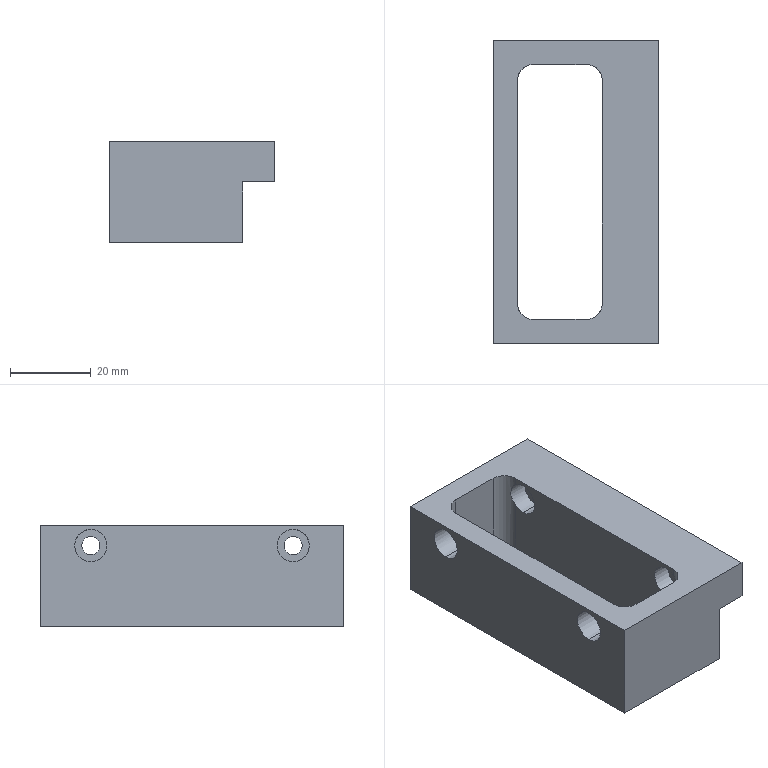Part | STEP file | X77-08305 | 1 solid | 39 faces | box 41 x 75 x 25 mm | volume 32721 mm3 | cylinder 20 | plane 19 | commonest cylinder face diameters 8 x16 4.5 x4
STEP:
#1=CARTESIAN_POINT('',(-3444.198,-146.809,24.));
#2=VERTEX_POINT('',#1);
#3=CARTESIAN_POINT('',(-3444.198,-146.809,16.));
#4=VERTEX_POINT('',#3);
#5=CARTESIAN_POINT('',(-3444.198,-146.809,20.));
#6=DIRECTION('',(1.,0.,0.));
#7=DIRECTION('',(0.,0.,-1.));
#8=AXIS2_PLACEMENT_3D('',#5,#6,#7);
#9=CIRCLE('',#8,4.);
#10=EDGE_CURVE('',#2,#4,#9,.T.);
#11=ORIENTED_EDGE('',*,*,#10,.T.);
#12=CARTESIAN_POINT('',(-3450.198,-146.809,16.));
#13=VERTEX_POINT('',#12);
#14=CARTESIAN_POINT('',(-3450.198,-146.809,16.));
#15=DIRECTION('',(-1.,0.,0.));
#16=VECTOR('',#15,1000.);
#17=LINE('',#14,#16);
#18=EDGE_CURVE('',#4,#13,#17,.T.);
#19=ORIENTED_EDGE('',*,*,#18,.T.);
#20=CARTESIAN_POINT('',(-3450.198,-146.809,24.));
#21=VERTEX_POINT('',#20);
#22=CARTESIAN_POINT('',(-3450.198,-146.809,20.));
#23=DIRECTION('',(-1.,0.,0.));
#24=DIRECTION('',(0.,0.,1.));
#25=AXIS2_PLACEMENT_3D('',#22,#23,#24);
#26=CIRCLE('',#25,4.);
#27=EDGE_CURVE('',#13,#21,#26,.T.);
#28=ORIENTED_EDGE('',*,*,#27,.T.);
#29=CARTESIAN_POINT('',(-3450.198,-146.809,24.));
#30=DIRECTION('',(-1.,0.,0.));
#31=VECTOR('',#30,1000.);
#32=LINE('',#29,#31);
#33=EDGE_CURVE('',#2,#21,#32,.T.);
#34=ORIENTED_EDGE('',*,*,#33,.F.);
#35=EDGE_LOOP('',(#11,#19,#28,#34));
#36=FACE_OUTER_BOUND('',#35,.T.);
#37=CARTESIAN_POINT('',(-3450.198,-146.809,20.));
#38=DIRECTION('',(-1.,0.,0.));
#39=DIRECTION('',(0.,0.,1.));
#40=AXIS2_PLACEMENT_3D('',#37,#38,#39);
#41=CYLINDRICAL_SURFACE('',#40,4.);
#42=ADVANCED_FACE('',(#36),#41,.F.);
#43=CARTESIAN_POINT('',(-3444.198,-199.309,16.878));
#44=VERTEX_POINT('',#43);
#45=CARTESIAN_POINT('',(-3444.198,-196.809,16.));
#46=VERTEX_POINT('',#45);
#47=CARTESIAN_POINT('',(-3444.198,-196.809,20.));
#48=DIRECTION('',(1.,0.,0.));
#49=DIRECTION('',(0.,0.,-1.));
#50=AXIS2_PLACEMENT_3D('',#47,#48,#49);
#51=CIRCLE('',#50,4.);
#52=EDGE_CURVE('',#44,#46,#51,.T.);
#53=ORIENTED_EDGE('',*,*,#52,.T.);
#54=CARTESIAN_POINT('',(-3450.198,-196.809,16.));
#55=VERTEX_POINT('',#54);
#56=CARTESIAN_POINT('',(-3450.198,-196.809,16.));
#57=DIRECTION('',(-1.,0.,0.));
#58=VECTOR('',#57,1000.);
#59=LINE('',#56,#58);
#60=EDGE_CURVE('',#46,#55,#59,.T.);
#61=ORIENTED_EDGE('',*,*,#60,.T.);
#62=CARTESIAN_POINT('',(-3450.198,-196.809,24.));
#63=VERTEX_POINT('',#62);
#64=CARTESIAN_POINT('',(-3450.198,-196.809,20.));
#65=DIRECTION('',(-1.,0.,0.));
#66=DIRECTION('',(0.,0.,1.));
#67=AXIS2_PLACEMENT_3D('',#64,#65,#66);
#68=CIRCLE('',#67,4.);
#69=EDGE_CURVE('',#55,#63,#68,.T.);
#70=ORIENTED_EDGE('',*,*,#69,.T.);
#71=CARTESIAN_POINT('',(-3444.198,-196.809,24.));
#72=VERTEX_POINT('',#71);
#73=CARTESIAN_POINT('',(-3450.198,-196.809,24.));
#74=DIRECTION('',(-1.,0.,0.));
#75=VECTOR('',#74,1000.);
#76=LINE('',#73,#75);
#77=EDGE_CURVE('',#72,#63,#76,.T.);
#78=ORIENTED_EDGE('',*,*,#77,.F.);
#79=CARTESIAN_POINT('',(-3444.198,-199.309,23.122));
#80=VERTEX_POINT('',#79);
#81=CARTESIAN_POINT('',(-3444.198,-196.809,20.));
#82=DIRECTION('',(1.,0.,0.));
#83=DIRECTION('',(0.,0.,-1.));
#84=AXIS2_PLACEMENT_3D('',#81,#82,#83);
#85=CIRCLE('',#84,4.);
#86=EDGE_CURVE('',#72,#80,#85,.T.);
#87=ORIENTED_EDGE('',*,*,#86,.T.);
#88=CARTESIAN_POINT('',(-3444.198,-199.309,23.122));
#89=CARTESIAN_POINT('',(-3444.198,-199.545,22.933));
#90=CARTESIAN_POINT('',(-3444.178,-199.755,22.722));
#91=CARTESIAN_POINT('',(-3444.119,-200.125,22.257));
#92=CARTESIAN_POINT('',(-3444.08,-200.285,22.));
#93=CARTESIAN_POINT('',(-3444.006,-200.542,21.466));
#94=CARTESIAN_POINT('',(-3443.971,-200.641,21.185));
#95=CARTESIAN_POINT('',(-3443.921,-200.775,20.599));
#96=CARTESIAN_POINT('',(-3443.907,-200.808,20.303));
#97=CARTESIAN_POINT('',(-3443.906,-200.809,19.706));
#98=CARTESIAN_POINT('',(-3443.921,-200.775,19.403));
#99=CARTESIAN_POINT('',(-3443.97,-200.643,18.823));
#100=CARTESIAN_POINT('',(-3444.005,-200.544,18.539));
#101=CARTESIAN_POINT('',(-3444.08,-200.286,18.001));
#102=CARTESIAN_POINT('',(-3444.118,-200.129,17.75));
#103=CARTESIAN_POINT('',(-3444.177,-199.759,17.282));
#104=CARTESIAN_POINT('',(-3444.198,-199.545,17.067));
#105=CARTESIAN_POINT('',(-3444.198,-199.309,16.878));
#106=B_SPLINE_CURVE_WITH_KNOTS('',3,(#88,#89,#90,#91,#92,#93,#94,#95,#96,#97,#98,#99,#100,#101,#102,#103,#104,#105),.UNSPECIFIED.,.F.,.F.,(4,2,2,2,2,2,2,2,4),(0.,0.0008939,0.001788,0.002682,0.003576,0.004469,0.005363,0.006257,0.007151),.UNSPECIFIED.);
#107=EDGE_CURVE('',#80,#44,#106,.T.);
#108=ORIENTED_EDGE('',*,*,#107,.T.);
#109=EDGE_LOOP('',(#53,#61,#70,#78,#87,#108));
#110=FACE_OUTER_BOUND('',#109,.T.);
#111=CARTESIAN_POINT('',(-3450.198,-196.809,20.));
#112=DIRECTION('',(-1.,0.,0.));
#113=DIRECTION('',(0.,0.,1.));
#114=AXIS2_PLACEMENT_3D('',#111,#112,#113);
#115=CYLINDRICAL_SURFACE('',#114,4.);
#116=ADVANCED_FACE('',(#110),#115,.F.);
#117=CARTESIAN_POINT('',(-3418.598,-146.809,16.));
#118=VERTEX_POINT('',#117);
#119=CARTESIAN_POINT('',(-3418.598,-146.809,24.));
#120=VERTEX_POINT('',#119);
#121=CARTESIAN_POINT('',(-3418.598,-146.809,20.));
#122=DIRECTION('',(-1.,0.,0.));
#123=DIRECTION('',(0.,0.,1.));
#124=AXIS2_PLACEMENT_3D('',#121,#122,#123);
#125=CIRCLE('',#124,4.);
#126=EDGE_CURVE('',#118,#120,#125,.T.);
#127=ORIENTED_EDGE('',*,*,#126,.F.);
#128=CARTESIAN_POINT('',(-3423.198,-146.809,16.));
#129=VERTEX_POINT('',#128);
#130=CARTESIAN_POINT('',(-3423.198,-146.809,16.));
#131=DIRECTION('',(-1.,0.,0.));
#132=VECTOR('',#131,1000.);
#133=LINE('',#130,#132);
#134=EDGE_CURVE('',#118,#129,#133,.T.);
#135=ORIENTED_EDGE('',*,*,#134,.T.);
#136=CARTESIAN_POINT('',(-3423.198,-146.809,24.));
#137=VERTEX_POINT('',#136);
#138=CARTESIAN_POINT('',(-3423.198,-146.809,20.));
#139=DIRECTION('',(-1.,0.,0.));
#140=DIRECTION('',(0.,0.,1.));
#141=AXIS2_PLACEMENT_3D('',#138,#139,#140);
#142=CIRCLE('',#141,4.);
#143=EDGE_CURVE('',#129,#137,#142,.T.);
#144=ORIENTED_EDGE('',*,*,#143,.T.);
#145=CARTESIAN_POINT('',(-3423.198,-146.809,24.));
#146=DIRECTION('',(-1.,0.,0.));
#147=VECTOR('',#146,1000.);
#148=LINE('',#145,#147);
#149=EDGE_CURVE('',#120,#137,#148,.T.);
#150=ORIENTED_EDGE('',*,*,#149,.F.);
#151=EDGE_LOOP('',(#127,#135,#144,#150));
#152=FACE_OUTER_BOUND('',#151,.T.);
#153=CARTESIAN_POINT('',(-3423.198,-146.809,20.));
#154=DIRECTION('',(-1.,0.,0.));
#155=DIRECTION('',(0.,0.,1.));
#156=AXIS2_PLACEMENT_3D('',#153,#154,#155);
#157=CYLINDRICAL_SURFACE('',#156,4.);
#158=ADVANCED_FACE('',(#152),#157,.F.);
#159=CARTESIAN_POINT('',(-3409.198,-146.809,22.25));
#160=VERTEX_POINT('',#159);
#161=CARTESIAN_POINT('',(-3409.198,-146.809,17.75));
#162=VERTEX_POINT('',#161);
#163=CARTESIAN_POINT('',(-3409.198,-146.809,20.));
#164=DIRECTION('',(1.,0.,0.));
#165=DIRECTION('',(0.,0.,-1.));
#166=AXIS2_PLACEMENT_3D('',#163,#164,#165);
#167=CIRCLE('',#166,2.25);
#168=EDGE_CURVE('',#160,#162,#167,.T.);
#169=ORIENTED_EDGE('',*,*,#168,.T.);
#170=CARTESIAN_POINT('',(-3418.598,-146.809,17.75));
#171=VERTEX_POINT('',#170);
#172=CARTESIAN_POINT('',(-3423.198,-146.809,17.75));
#173=DIRECTION('',(-1.,0.,0.));
#174=VECTOR('',#173,1000.);
#175=LINE('',#172,#174);
#176=EDGE_CURVE('',#162,#171,#175,.T.);
#177=ORIENTED_EDGE('',*,*,#176,.T.);
#178=CARTESIAN_POINT('',(-3418.598,-146.809,22.25));
#179=VERTEX_POINT('',#178);
#180=CARTESIAN_POINT('',(-3418.598,-146.809,20.));
#181=DIRECTION('',(-1.,0.,0.));
#182=DIRECTION('',(0.,0.,1.));
#183=AXIS2_PLACEMENT_3D('',#180,#181,#182);
#184=CIRCLE('',#183,2.25);
#185=EDGE_CURVE('',#171,#179,#184,.T.);
#186=ORIENTED_EDGE('',*,*,#185,.T.);
#187=CARTESIAN_POINT('',(-3423.198,-146.809,22.25));
#188=DIRECTION('',(-1.,0.,0.));
#189=VECTOR('',#188,1000.);
#190=LINE('',#187,#189);
#191=EDGE_CURVE('',#160,#179,#190,.T.);
#192=ORIENTED_EDGE('',*,*,#191,.F.);
#193=EDGE_LOOP('',(#169,#177,#186,#192));
#194=FACE_OUTER_BOUND('',#193,.T.);
#195=CARTESIAN_POINT('',(-3423.198,-146.809,20.));
#196=DIRECTION('',(-1.,0.,0.));
#197=DIRECTION('',(0.,0.,1.));
#198=AXIS2_PLACEMENT_3D('',#195,#196,#197);
#199=CYLINDRICAL_SURFACE('',#198,2.25);
#200=ADVANCED_FACE('',(#194),#199,.F.);
#201=CARTESIAN_POINT('',(-3418.598,-196.809,16.));
#202=VERTEX_POINT('',#201);
#203=CARTESIAN_POINT('',(-3418.598,-196.809,24.));
#204=VERTEX_POINT('',#203);
#205=CARTESIAN_POINT('',(-3418.598,-196.809,20.));
#206=DIRECTION('',(-1.,0.,0.));
#207=DIRECTION('',(0.,0.,1.));
#208=AXIS2_PLACEMENT_3D('',#205,#206,#207);
#209=CIRCLE('',#208,4.);
#210=EDGE_CURVE('',#202,#204,#209,.T.);
#211=ORIENTED_EDGE('',*,*,#210,.F.);
#212=CARTESIAN_POINT('',(-3423.198,-196.809,16.));
#213=VERTEX_POINT('',#212);
#214=CARTESIAN_POINT('',(-3423.198,-196.809,16.));
#215=DIRECTION('',(-1.,0.,0.));
#216=VECTOR('',#215,1000.);
#217=LINE('',#214,#216);
#218=EDGE_CURVE('',#202,#213,#217,.T.);
#219=ORIENTED_EDGE('',*,*,#218,.T.);
#220=CARTESIAN_POINT('',(-3423.198,-199.309,16.878));
#221=VERTEX_POINT('',#220);
#222=CARTESIAN_POINT('',(-3423.198,-196.809,20.));
#223=DIRECTION('',(-1.,0.,0.));
#224=DIRECTION('',(0.,0.,1.));
#225=AXIS2_PLACEMENT_3D('',#222,#223,#224);
#226=CIRCLE('',#225,4.);
#227=EDGE_CURVE('',#213,#221,#226,.T.);
#228=ORIENTED_EDGE('',*,*,#227,.T.);
#229=CARTESIAN_POINT('',(-3423.198,-199.309,23.122));
#230=VERTEX_POINT('',#229);
#231=CARTESIAN_POINT('',(-3423.198,-199.309,23.122));
#232=CARTESIAN_POINT('',(-3423.198,-199.545,22.933));
#233=CARTESIAN_POINT('',(-3423.219,-199.755,22.722));
#234=CARTESIAN_POINT('',(-3423.278,-200.125,22.257));
#235=CARTESIAN_POINT('',(-3423.317,-200.285,22.));
#236=CARTESIAN_POINT('',(-3423.391,-200.542,21.466));
#237=CARTESIAN_POINT('',(-3423.426,-200.641,21.185));
#238=CARTESIAN_POINT('',(-3423.476,-200.775,20.599));
#239=CARTESIAN_POINT('',(-3423.49,-200.808,20.303));
#240=CARTESIAN_POINT('',(-3423.491,-200.809,19.706));
#241=CARTESIAN_POINT('',(-3423.476,-200.775,19.403));
#242=CARTESIAN_POINT('',(-3423.427,-200.643,18.823));
#243=CARTESIAN_POINT('',(-3423.392,-200.544,18.539));
#244=CARTESIAN_POINT('',(-3423.317,-200.286,18.001));
#245=CARTESIAN_POINT('',(-3423.279,-200.129,17.75));
#246=CARTESIAN_POINT('',(-3423.219,-199.759,17.282));
#247=CARTESIAN_POINT('',(-3423.198,-199.545,17.067));
#248=CARTESIAN_POINT('',(-3423.198,-199.309,16.878));
#249=B_SPLINE_CURVE_WITH_KNOTS('',3,(#231,#232,#233,#234,#235,#236,#237,#238,#239,#240,#241,#242,#243,#244,#245,#246,#247,#248),.UNSPECIFIED.,.F.,.F.,(4,2,2,2,2,2,2,2,4),(0.,0.0008939,0.001788,0.002682,0.003576,0.004469,0.005363,0.006257,0.007151),.UNSPECIFIED.);
#250=EDGE_CURVE('',#230,#221,#249,.T.);
#251=ORIENTED_EDGE('',*,*,#250,.F.);
#252=CARTESIAN_POINT('',(-3423.198,-196.809,24.));
#253=VERTEX_POINT('',#252);
#254=CARTESIAN_POINT('',(-3423.198,-196.809,20.));
#255=DIRECTION('',(-1.,0.,0.));
#256=DIRECTION('',(0.,0.,1.));
#257=AXIS2_PLACEMENT_3D('',#254,#255,#256);
#258=CIRCLE('',#257,4.);
#259=EDGE_CURVE('',#230,#253,#258,.T.);
#260=ORIENTED_EDGE('',*,*,#259,.T.);
#261=CARTESIAN_POINT('',(-3423.198,-196.809,24.));
#262=DIRECTION('',(-1.,0.,0.));
#263=VECTOR('',#262,1000.);
#264=LINE('',#261,#263);
#265=EDGE_CURVE('',#204,#253,#264,.T.);
#266=ORIENTED_EDGE('',*,*,#265,.F.);
#267=EDGE_LOOP('',(#211,#219,#228,#251,#260,#266));
#268=FACE_OUTER_BOUND('',#267,.T.);
#269=CARTESIAN_POINT('',(-3423.198,-196.809,20.));
#270=DIRECTION('',(-1.,0.,0.));
#271=DIRECTION('',(0.,0.,1.));
#272=AXIS2_PLACEMENT_3D('',#269,#270,#271);
#273=CYLINDRICAL_SURFACE('',#272,4.);
#274=ADVANCED_FACE('',(#268),#273,.F.);
#275=CARTESIAN_POINT('',(-3409.198,-196.809,22.25));
#276=VERTEX_POINT('',#275);
#277=CARTESIAN_POINT('',(-3409.198,-196.809,17.75));
#278=VERTEX_POINT('',#277);
#279=CARTESIAN_POINT('',(-3409.198,-196.809,20.));
#280=DIRECTION('',(1.,0.,0.));
#281=DIRECTION('',(0.,0.,-1.));
#282=AXIS2_PLACEMENT_3D('',#279,#280,#281);
#283=CIRCLE('',#282,2.25);
#284=EDGE_CURVE('',#276,#278,#283,.T.);
#285=ORIENTED_EDGE('',*,*,#284,.T.);
#286=CARTESIAN_POINT('',(-3418.598,-196.809,17.75));
#287=VERTEX_POINT('',#286);
#288=CARTESIAN_POINT('',(-3423.198,-196.809,17.75));
#289=DIRECTION('',(-1.,0.,0.));
#290=VECTOR('',#289,1000.);
#291=LINE('',#288,#290);
#292=EDGE_CURVE('',#278,#287,#291,.T.);
#293=ORIENTED_EDGE('',*,*,#292,.T.);
#294=CARTESIAN_POINT('',(-3418.598,-196.809,22.25));
#295=VERTEX_POINT('',#294);
#296=CARTESIAN_POINT('',(-3418.598,-196.809,20.));
#297=DIRECTION('',(-1.,0.,0.));
#298=DIRECTION('',(0.,0.,1.));
#299=AXIS2_PLACEMENT_3D('',#296,#297,#298);
#300=CIRCLE('',#299,2.25);
#301=EDGE_CURVE('',#287,#295,#300,.T.);
#302=ORIENTED_EDGE('',*,*,#301,.T.);
#303=CARTESIAN_POINT('',(-3423.198,-196.809,22.25));
#304=DIRECTION('',(-1.,0.,0.));
#305=VECTOR('',#304,1000.);
#306=LINE('',#303,#305);
#307=EDGE_CURVE('',#276,#295,#306,.T.);
#308=ORIENTED_EDGE('',*,*,#307,.F.);
#309=EDGE_LOOP('',(#285,#293,#302,#308));
#310=FACE_OUTER_BOUND('',#309,.T.);
#311=CARTESIAN_POINT('',(-3423.198,-196.809,20.));
#312=DIRECTION('',(-1.,0.,0.));
#313=DIRECTION('',(0.,0.,1.));
#314=AXIS2_PLACEMENT_3D('',#311,#312,#313);
#315=CYLINDRICAL_SURFACE('',#314,2.25);
#316=ADVANCED_FACE('',(#310),#315,.F.);
#317=CARTESIAN_POINT('',(-3417.198,-209.309,15.));
#318=VERTEX_POINT('',#317);
#319=CARTESIAN_POINT('',(-3417.198,-134.309,15.));
#320=VERTEX_POINT('',#319);
#321=CARTESIAN_POINT('',(-3417.198,-134.309,15.));
#322=DIRECTION('',(0.,1.,0.));
#323=VECTOR('',#322,1000.);
#324=LINE('',#321,#323);
#325=EDGE_CURVE('',#318,#320,#324,.T.);
#326=ORIENTED_EDGE('',*,*,#325,.F.);
#327=CARTESIAN_POINT('',(-3417.198,-209.309,0.));
#328=VERTEX_POINT('',#327);
#329=CARTESIAN_POINT('',(-3417.198,-209.309,25.));
#330=DIRECTION('',(0.,0.,-1.));
#331=VECTOR('',#330,1000.);
#332=LINE('',#329,#331);
#333=EDGE_CURVE('',#318,#328,#332,.T.);
#334=ORIENTED_EDGE('',*,*,#333,.T.);
#335=CARTESIAN_POINT('',(-3417.198,-134.309,0.));
#336=VERTEX_POINT('',#335);
#337=CARTESIAN_POINT('',(-3417.198,-209.309,0.));
#338=DIRECTION('',(0.,1.,0.));
#339=VECTOR('',#338,1000.);
#340=LINE('',#337,#339);
#341=EDGE_CURVE('',#328,#336,#340,.T.);
#342=ORIENTED_EDGE('',*,*,#341,.T.);
#343=CARTESIAN_POINT('',(-3417.198,-134.309,25.));
#344=DIRECTION('',(0.,0.,-1.));
#345=VECTOR('',#344,1000.);
#346=LINE('',#343,#345);
#347=EDGE_CURVE('',#320,#336,#346,.T.);
#348=ORIENTED_EDGE('',*,*,#347,.F.);
#349=EDGE_LOOP('',(#326,#334,#342,#348));
#350=FACE_OUTER_BOUND('',#349,.T.);
#351=CARTESIAN_POINT('',(-3417.198,-209.309,25.));
#352=DIRECTION('',(-1.,0.,0.));
#353=DIRECTION('',(0.,0.,1.));
#354=AXIS2_PLACEMENT_3D('',#351,#352,#353);
#355=PLANE('',#354);
#356=ADVANCED_FACE('',(#350),#355,.F.);
#357=CARTESIAN_POINT('',(-3450.198,-134.309,25.));
#358=VERTEX_POINT('',#357);
#359=CARTESIAN_POINT('',(-3450.198,-209.309,25.));
#360=VERTEX_POINT('',#359);
#361=CARTESIAN_POINT('',(-3450.198,-209.309,25.));
#362=DIRECTION('',(0.,-1.,0.));
#363=VECTOR('',#362,1000.);
#364=LINE('',#361,#363);
#365=EDGE_CURVE('',#358,#360,#364,.T.);
#366=ORIENTED_EDGE('',*,*,#365,.T.);
#367=CARTESIAN_POINT('',(-3409.198,-209.309,25.));
#368=VERTEX_POINT('',#367);
#369=CARTESIAN_POINT('',(-3417.198,-209.309,25.));
#370=DIRECTION('',(1.,0.,0.));
#371=VECTOR('',#370,1000.);
#372=LINE('',#369,#371);
#373=EDGE_CURVE('',#360,#368,#372,.T.);
#374=ORIENTED_EDGE('',*,*,#373,.T.);
#375=CARTESIAN_POINT('',(-3409.198,-134.309,25.));
#376=VERTEX_POINT('',#375);
#377=CARTESIAN_POINT('',(-3409.198,-134.309,25.));
#378=DIRECTION('',(0.,-1.,0.));
#379=VECTOR('',#378,1000.);
#380=LINE('',#377,#379);
#381=EDGE_CURVE('',#376,#368,#380,.T.);
#382=ORIENTED_EDGE('',*,*,#381,.F.);
#383=CARTESIAN_POINT('',(-3417.198,-134.309,25.));
#384=DIRECTION('',(-1.,0.,0.));
#385=VECTOR('',#384,1000.);
#386=LINE('',#383,#385);
#387=EDGE_CURVE('',#376,#358,#386,.T.);
#388=ORIENTED_EDGE('',*,*,#387,.T.);
#389=EDGE_LOOP('',(#366,#374,#382,#388));
#390=FACE_OUTER_BOUND('',#389,.T.);
#391=CARTESIAN_POINT('',(-3423.198,-199.309,25.));
#392=VERTEX_POINT('',#391);
#393=CARTESIAN_POINT('',(-3423.198,-144.309,25.));
#394=VERTEX_POINT('',#393);
#395=CARTESIAN_POINT('',(-3423.198,-199.309,25.));
#396=DIRECTION('',(0.,1.,0.));
#397=VECTOR('',#396,1000.);
#398=LINE('',#395,#397);
#399=EDGE_CURVE('',#392,#394,#398,.T.);
#400=ORIENTED_EDGE('',*,*,#399,.F.);
#401=CARTESIAN_POINT('',(-3427.198,-203.309,25.));
#402=VERTEX_POINT('',#401);
#403=CARTESIAN_POINT('',(-3427.198,-199.309,25.));
#404=DIRECTION('',(0.,0.,1.));
#405=DIRECTION('',(1.,0.,0.));
#406=AXIS2_PLACEMENT_3D('',#403,#404,#405);
#407=CIRCLE('',#406,4.);
#408=EDGE_CURVE('',#402,#392,#407,.T.);
#409=ORIENTED_EDGE('',*,*,#408,.F.);
#410=CARTESIAN_POINT('',(-3440.198,-203.309,25.));
#411=VERTEX_POINT('',#410);
#412=CARTESIAN_POINT('',(-3427.198,-203.309,25.));
#413=DIRECTION('',(1.,0.,0.));
#414=VECTOR('',#413,1000.);
#415=LINE('',#412,#414);
#416=EDGE_CURVE('',#411,#402,#415,.T.);
#417=ORIENTED_EDGE('',*,*,#416,.F.);
#418=CARTESIAN_POINT('',(-3444.198,-199.309,25.));
#419=VERTEX_POINT('',#418);
#420=CARTESIAN_POINT('',(-3440.198,-199.309,25.));
#421=DIRECTION('',(0.,0.,1.));
#422=DIRECTION('',(-1.,0.,0.));
#423=AXIS2_PLACEMENT_3D('',#420,#421,#422);
#424=CIRCLE('',#423,4.);
#425=EDGE_CURVE('',#419,#411,#424,.T.);
#426=ORIENTED_EDGE('',*,*,#425,.F.);
#427=CARTESIAN_POINT('',(-3444.198,-144.309,25.));
#428=VERTEX_POINT('',#427);
#429=CARTESIAN_POINT('',(-3444.198,-199.309,25.));
#430=DIRECTION('',(0.,-1.,0.));
#431=VECTOR('',#430,1000.);
#432=LINE('',#429,#431);
#433=EDGE_CURVE('',#428,#419,#432,.T.);
#434=ORIENTED_EDGE('',*,*,#433,.F.);
#435=CARTESIAN_POINT('',(-3440.198,-140.309,25.));
#436=VERTEX_POINT('',#435);
#437=CARTESIAN_POINT('',(-3440.198,-144.309,25.));
#438=DIRECTION('',(0.,0.,1.));
#439=DIRECTION('',(1.,0.,0.));
#440=AXIS2_PLACEMENT_3D('',#437,#438,#439);
#441=CIRCLE('',#440,4.);
#442=EDGE_CURVE('',#436,#428,#441,.T.);
#443=ORIENTED_EDGE('',*,*,#442,.F.);
#444=CARTESIAN_POINT('',(-3427.198,-140.309,25.));
#445=VERTEX_POINT('',#444);
#446=CARTESIAN_POINT('',(-3427.198,-140.309,25.));
#447=DIRECTION('',(-1.,0.,0.));
#448=VECTOR('',#447,1000.);
#449=LINE('',#446,#448);
#450=EDGE_CURVE('',#445,#436,#449,.T.);
#451=ORIENTED_EDGE('',*,*,#450,.F.);
#452=CARTESIAN_POINT('',(-3427.198,-144.309,25.));
#453=DIRECTION('',(0.,0.,1.));
#454=DIRECTION('',(1.,0.,0.));
#455=AXIS2_PLACEMENT_3D('',#452,#453,#454);
#456=CIRCLE('',#455,4.);
#457=EDGE_CURVE('',#394,#445,#456,.T.);
#458=ORIENTED_EDGE('',*,*,#457,.F.);
#459=EDGE_LOOP('',(#400,#409,#417,#426,#434,#443,#451,#458));
#460=FACE_BOUND('',#459,.T.);
#461=CARTESIAN_POINT('',(-3450.198,-134.309,25.));
#462=DIRECTION('',(0.,0.,1.));
#463=DIRECTION('',(1.,0.,0.));
#464=AXIS2_PLACEMENT_3D('',#461,#462,#463);
#465=PLANE('',#464);
#466=ADVANCED_FACE('',(#390,#460),#465,.T.);
#467=CARTESIAN_POINT('',(-3446.198,-201.309,0.));
#468=VERTEX_POINT('',#467);
#469=CARTESIAN_POINT('',(-3446.198,-142.309,0.));
#470=VERTEX_POINT('',#469);
#471=CARTESIAN_POINT('',(-3446.198,-201.309,0.));
#472=DIRECTION('',(0.,1.,0.));
#473=VECTOR('',#472,1000.);
#474=LINE('',#471,#473);
#475=EDGE_CURVE('',#468,#470,#474,.T.);
#476=ORIENTED_EDGE('',*,*,#475,.F.);
#477=CARTESIAN_POINT('',(-3442.198,-205.309,0.));
#478=VERTEX_POINT('',#477);
#479=CARTESIAN_POINT('',(-3442.198,-201.309,0.));
#480=DIRECTION('',(0.,0.,-1.));
#481=DIRECTION('',(1.,0.,0.));
#482=AXIS2_PLACEMENT_3D('',#479,#480,#481);
#483=CIRCLE('',#482,4.);
#484=EDGE_CURVE('',#478,#468,#483,.T.);
#485=ORIENTED_EDGE('',*,*,#484,.F.);
#486=CARTESIAN_POINT('',(-3425.198,-205.309,0.));
#487=VERTEX_POINT('',#486);
#488=CARTESIAN_POINT('',(-3425.198,-205.309,0.));
#489=DIRECTION('',(-1.,0.,0.));
#490=VECTOR('',#489,1000.);
#491=LINE('',#488,#490);
#492=EDGE_CURVE('',#487,#478,#491,.T.);
#493=ORIENTED_EDGE('',*,*,#492,.F.);
#494=CARTESIAN_POINT('',(-3421.198,-201.309,0.));
#495=VERTEX_POINT('',#494);
#496=CARTESIAN_POINT('',(-3425.198,-201.309,0.));
#497=DIRECTION('',(0.,0.,-1.));
#498=DIRECTION('',(1.,0.,0.));
#499=AXIS2_PLACEMENT_3D('',#496,#497,#498);
#500=CIRCLE('',#499,4.);
#501=EDGE_CURVE('',#495,#487,#500,.T.);
#502=ORIENTED_EDGE('',*,*,#501,.F.);
#503=CARTESIAN_POINT('',(-3421.198,-142.309,0.));
#504=VERTEX_POINT('',#503);
#505=CARTESIAN_POINT('',(-3421.198,-142.309,0.));
#506=DIRECTION('',(0.,-1.,0.));
#507=VECTOR('',#506,1000.);
#508=LINE('',#505,#507);
#509=EDGE_CURVE('',#504,#495,#508,.T.);
#510=ORIENTED_EDGE('',*,*,#509,.F.);
#511=CARTESIAN_POINT('',(-3425.198,-138.309,0.));
#512=VERTEX_POINT('',#511);
#513=CARTESIAN_POINT('',(-3425.198,-142.309,0.));
#514=DIRECTION('',(0.,0.,-1.));
#515=DIRECTION('',(-1.,0.,0.));
#516=AXIS2_PLACEMENT_3D('',#513,#514,#515);
#517=CIRCLE('',#516,4.);
#518=EDGE_CURVE('',#512,#504,#517,.T.);
#519=ORIENTED_EDGE('',*,*,#518,.F.);
#520=CARTESIAN_POINT('',(-3442.198,-138.309,0.));
#521=VERTEX_POINT('',#520);
#522=CARTESIAN_POINT('',(-3442.198,-138.309,0.));
#523=DIRECTION('',(1.,0.,0.));
#524=VECTOR('',#523,1000.);
#525=LINE('',#522,#524);
#526=EDGE_CURVE('',#521,#512,#525,.T.);
#527=ORIENTED_EDGE('',*,*,#526,.F.);
#528=CARTESIAN_POINT('',(-3442.198,-142.309,0.));
#529=DIRECTION('',(0.,0.,-1.));
#530=DIRECTION('',(-1.,0.,0.));
#531=AXIS2_PLACEMENT_3D('',#528,#529,#530);
#532=CIRCLE('',#531,4.);
#533=EDGE_CURVE('',#470,#521,#532,.T.);
#534=ORIENTED_EDGE('',*,*,#533,.F.);
#535=EDGE_LOOP('',(#476,#485,#493,#502,#510,#519,#527,#534));
#536=FACE_BOUND('',#535,.T.);
#537=CARTESIAN_POINT('',(-3450.198,-134.309,0.));
#538=VERTEX_POINT('',#537);
#539=CARTESIAN_POINT('',(-3450.198,-209.309,0.));
#540=VERTEX_POINT('',#539);
#541=CARTESIAN_POINT('',(-3450.198,-209.309,0.));
#542=DIRECTION('',(0.,-1.,0.));
#543=VECTOR('',#542,1000.);
#544=LINE('',#541,#543);
#545=EDGE_CURVE('',#538,#540,#544,.T.);
#546=ORIENTED_EDGE('',*,*,#545,.F.);
#547=CARTESIAN_POINT('',(-3417.198,-134.309,0.));
#548=DIRECTION('',(-1.,0.,0.));
#549=VECTOR('',#548,1000.);
#550=LINE('',#547,#549);
#551=EDGE_CURVE('',#336,#538,#550,.T.);
#552=ORIENTED_EDGE('',*,*,#551,.F.);
#553=ORIENTED_EDGE('',*,*,#341,.F.);
#554=CARTESIAN_POINT('',(-3417.198,-209.309,0.));
#555=DIRECTION('',(1.,0.,0.));
#556=VECTOR('',#555,1000.);
#557=LINE('',#554,#556);
#558=EDGE_CURVE('',#540,#328,#557,.T.);
#559=ORIENTED_EDGE('',*,*,#558,.F.);
#560=EDGE_LOOP('',(#546,#552,#553,#559));
#561=FACE_OUTER_BOUND('',#560,.T.);
#562=CARTESIAN_POINT('',(-3450.198,-134.309,0.));
#563=DIRECTION('',(0.,0.,1.));
#564=DIRECTION('',(1.,0.,0.));
#565=AXIS2_PLACEMENT_3D('',#562,#563,#564);
#566=PLANE('',#565);
#567=ADVANCED_FACE('',(#536,#561),#566,.F.);
#568=CARTESIAN_POINT('',(-3450.198,-146.809,20.));
#569=DIRECTION('',(-1.,0.,0.));
#570=DIRECTION('',(0.,0.,1.));
#571=AXIS2_PLACEMENT_3D('',#568,#569,#570);
#572=CIRCLE('',#571,4.);
#573=EDGE_CURVE('',#21,#13,#572,.T.);
#574=ORIENTED_EDGE('',*,*,#573,.F.);
#575=ORIENTED_EDGE('',*,*,#27,.F.);
#576=EDGE_LOOP('',(#574,#575));
#577=FACE_BOUND('',#576,.T.);
#578=CARTESIAN_POINT('',(-3450.198,-196.809,20.));
#579=DIRECTION('',(-1.,0.,0.));
#580=DIRECTION('',(0.,0.,1.));
#581=AXIS2_PLACEMENT_3D('',#578,#579,#580);
#582=CIRCLE('',#581,4.);
#583=EDGE_CURVE('',#63,#55,#582,.T.);
#584=ORIENTED_EDGE('',*,*,#583,.F.);
#585=ORIENTED_EDGE('',*,*,#69,.F.);
#586=EDGE_LOOP('',(#584,#585));
#587=FACE_BOUND('',#586,.T.);
#588=ORIENTED_EDGE('',*,*,#545,.T.);
#589=CARTESIAN_POINT('',(-3450.198,-209.309,25.));
#590=DIRECTION('',(0.,0.,-1.));
#591=VECTOR('',#590,1000.);
#592=LINE('',#589,#591);
#593=EDGE_CURVE('',#360,#540,#592,.T.);
#594=ORIENTED_EDGE('',*,*,#593,.F.);
#595=ORIENTED_EDGE('',*,*,#365,.F.);
#596=CARTESIAN_POINT('',(-3450.198,-134.309,25.));
#597=DIRECTION('',(0.,0.,-1.));
#598=VECTOR('',#597,1000.);
#599=LINE('',#596,#598);
#600=EDGE_CURVE('',#358,#538,#599,.T.);
#601=ORIENTED_EDGE('',*,*,#600,.T.);
#602=EDGE_LOOP('',(#588,#594,#595,#601));
#603=FACE_OUTER_BOUND('',#602,.T.);
#604=CARTESIAN_POINT('',(-3450.198,-209.309,25.));
#605=DIRECTION('',(1.,0.,0.));
#606=DIRECTION('',(0.,0.,-1.));
#607=AXIS2_PLACEMENT_3D('',#604,#605,#606);
#608=PLANE('',#607);
#609=ADVANCED_FACE('',(#577,#587,#603),#608,.F.);
#610=ORIENTED_EDGE('',*,*,#558,.T.);
#611=ORIENTED_EDGE('',*,*,#333,.F.);
#612=CARTESIAN_POINT('',(-3409.198,-209.309,15.));
#613=VERTEX_POINT('',#612);
#614=CARTESIAN_POINT('',(-3409.198,-209.309,15.));
#615=DIRECTION('',(-1.,0.,0.));
#616=VECTOR('',#615,1000.);
#617=LINE('',#614,#616);
#618=EDGE_CURVE('',#613,#318,#617,.T.);
#619=ORIENTED_EDGE('',*,*,#618,.F.);
#620=CARTESIAN_POINT('',(-3409.198,-209.309,25.));
#621=DIRECTION('',(0.,0.,-1.));
#622=VECTOR('',#621,1000.);
#623=LINE('',#620,#622);
#624=EDGE_CURVE('',#368,#613,#623,.T.);
#625=ORIENTED_EDGE('',*,*,#624,.F.);
#626=ORIENTED_EDGE('',*,*,#373,.F.);
#627=ORIENTED_EDGE('',*,*,#593,.T.);
#628=EDGE_LOOP('',(#610,#611,#619,#625,#626,#627));
#629=FACE_OUTER_BOUND('',#628,.T.);
#630=CARTESIAN_POINT('',(-3417.198,-209.309,25.));
#631=DIRECTION('',(0.,1.,0.));
#632=DIRECTION('',(0.,0.,1.));
#633=AXIS2_PLACEMENT_3D('',#630,#631,#632);
#634=PLANE('',#633);
#635=ADVANCED_FACE('',(#629),#634,.F.);
#636=ORIENTED_EDGE('',*,*,#551,.T.);
#637=ORIENTED_EDGE('',*,*,#600,.F.);
#638=ORIENTED_EDGE('',*,*,#387,.F.);
#639=CARTESIAN_POINT('',(-3409.198,-134.309,15.));
#640=VERTEX_POINT('',#639);
#641=CARTESIAN_POINT('',(-3409.198,-134.309,25.));
#642=DIRECTION('',(0.,0.,1.));
#643=VECTOR('',#642,1000.);
#644=LINE('',#641,#643);
#645=EDGE_CURVE('',#640,#376,#644,.T.);
#646=ORIENTED_EDGE('',*,*,#645,.F.);
#647=CARTESIAN_POINT('',(-3409.198,-134.309,15.));
#648=DIRECTION('',(-1.,0.,0.));
#649=VECTOR('',#648,1000.);
#650=LINE('',#647,#649);
#651=EDGE_CURVE('',#640,#320,#650,.T.);
#652=ORIENTED_EDGE('',*,*,#651,.T.);
#653=ORIENTED_EDGE('',*,*,#347,.T.);
#654=EDGE_LOOP('',(#636,#637,#638,#646,#652,#653));
#655=FACE_OUTER_BOUND('',#654,.T.);
#656=CARTESIAN_POINT('',(-3417.198,-134.309,25.));
#657=DIRECTION('',(0.,-1.,0.));
#658=DIRECTION('',(0.,0.,-1.));
#659=AXIS2_PLACEMENT_3D('',#656,#657,#658);
#660=PLANE('',#659);
#661=ADVANCED_FACE('',(#655),#660,.F.);
#662=CARTESIAN_POINT('',(-3427.198,-203.309,3.));
#663=VERTEX_POINT('',#662);
#664=CARTESIAN_POINT('',(-3423.198,-199.309,3.));
#665=VERTEX_POINT('',#664);
#666=CARTESIAN_POINT('',(-3427.198,-199.309,3.));
#667=DIRECTION('',(0.,0.,1.));
#668=DIRECTION('',(1.,0.,0.));
#669=AXIS2_PLACEMENT_3D('',#666,#667,#668);
#670=CIRCLE('',#669,4.);
#671=EDGE_CURVE('',#663,#665,#670,.T.);
#672=ORIENTED_EDGE('',*,*,#671,.F.);
#673=CARTESIAN_POINT('',(-3427.198,-203.309,25.));
#674=DIRECTION('',(0.,0.,-1.));
#675=VECTOR('',#674,1000.);
#676=LINE('',#673,#675);
#677=EDGE_CURVE('',#402,#663,#676,.T.);
#678=ORIENTED_EDGE('',*,*,#677,.F.);
#679=ORIENTED_EDGE('',*,*,#408,.T.);
#680=CARTESIAN_POINT('',(-3423.198,-199.309,25.));
#681=DIRECTION('',(0.,0.,-1.));
#682=VECTOR('',#681,1000.);
#683=LINE('',#680,#682);
#684=EDGE_CURVE('',#392,#230,#683,.T.);
#685=ORIENTED_EDGE('',*,*,#684,.T.);
#686=ORIENTED_EDGE('',*,*,#250,.T.);
#687=CARTESIAN_POINT('',(-3423.198,-199.309,25.));
#688=DIRECTION('',(0.,0.,-1.));
#689=VECTOR('',#688,1000.);
#690=LINE('',#687,#689);
#691=EDGE_CURVE('',#221,#665,#690,.T.);
#692=ORIENTED_EDGE('',*,*,#691,.T.);
#693=EDGE_LOOP('',(#672,#678,#679,#685,#686,#692));
#694=FACE_OUTER_BOUND('',#693,.T.);
#695=CARTESIAN_POINT('',(-3427.198,-199.309,25.));
#696=DIRECTION('',(0.,0.,-1.));
#697=DIRECTION('',(-1.,0.,0.));
#698=AXIS2_PLACEMENT_3D('',#695,#696,#697);
#699=CYLINDRICAL_SURFACE('',#698,4.);
#700=ADVANCED_FACE('',(#694),#699,.F.);
#701=CARTESIAN_POINT('',(-3423.198,-144.309,3.));
#702=VERTEX_POINT('',#701);
#703=CARTESIAN_POINT('',(-3423.198,-199.309,3.));
#704=DIRECTION('',(0.,1.,0.));
#705=VECTOR('',#704,1000.);
#706=LINE('',#703,#705);
#707=EDGE_CURVE('',#665,#702,#706,.T.);
#708=ORIENTED_EDGE('',*,*,#707,.F.);
#709=ORIENTED_EDGE('',*,*,#691,.F.);
#710=ORIENTED_EDGE('',*,*,#227,.F.);
#711=CARTESIAN_POINT('',(-3423.198,-196.809,20.));
#712=DIRECTION('',(-1.,0.,0.));
#713=DIRECTION('',(0.,0.,1.));
#714=AXIS2_PLACEMENT_3D('',#711,#712,#713);
#715=CIRCLE('',#714,4.);
#716=EDGE_CURVE('',#253,#213,#715,.T.);
#717=ORIENTED_EDGE('',*,*,#716,.F.);
#718=ORIENTED_EDGE('',*,*,#259,.F.);
#719=ORIENTED_EDGE('',*,*,#684,.F.);
#720=ORIENTED_EDGE('',*,*,#399,.T.);
#721=CARTESIAN_POINT('',(-3423.198,-144.309,23.122));
#722=VERTEX_POINT('',#721);
#723=CARTESIAN_POINT('',(-3423.198,-144.309,25.));
#724=DIRECTION('',(0.,0.,-1.));
#725=VECTOR('',#724,1000.);
#726=LINE('',#723,#725);
#727=EDGE_CURVE('',#394,#722,#726,.T.);
#728=ORIENTED_EDGE('',*,*,#727,.T.);
#729=CARTESIAN_POINT('',(-3423.198,-146.809,20.));
#730=DIRECTION('',(-1.,0.,0.));
#731=DIRECTION('',(0.,0.,1.));
#732=AXIS2_PLACEMENT_3D('',#729,#730,#731);
#733=CIRCLE('',#732,4.);
#734=EDGE_CURVE('',#137,#722,#733,.T.);
#735=ORIENTED_EDGE('',*,*,#734,.F.);
#736=ORIENTED_EDGE('',*,*,#143,.F.);
#737=CARTESIAN_POINT('',(-3423.198,-144.309,16.878));
#738=VERTEX_POINT('',#737);
#739=CARTESIAN_POINT('',(-3423.198,-146.809,20.));
#740=DIRECTION('',(-1.,0.,0.));
#741=DIRECTION('',(0.,0.,1.));
#742=AXIS2_PLACEMENT_3D('',#739,#740,#741);
#743=CIRCLE('',#742,4.);
#744=EDGE_CURVE('',#738,#129,#743,.T.);
#745=ORIENTED_EDGE('',*,*,#744,.F.);
#746=CARTESIAN_POINT('',(-3423.198,-144.309,25.));
#747=DIRECTION('',(0.,0.,-1.));
#748=VECTOR('',#747,1000.);
#749=LINE('',#746,#748);
#750=EDGE_CURVE('',#738,#702,#749,.T.);
#751=ORIENTED_EDGE('',*,*,#750,.T.);
#752=EDGE_LOOP('',(#708,#709,#710,#717,#718,#719,#720,#728,#735,#736,#745,#751));
#753=FACE_OUTER_BOUND('',#752,.T.);
#754=CARTESIAN_POINT('',(-3423.198,-199.309,25.));
#755=DIRECTION('',(-1.,0.,0.));
#756=DIRECTION('',(0.,0.,1.));
#757=AXIS2_PLACEMENT_3D('',#754,#755,#756);
#758=PLANE('',#757);
#759=ADVANCED_FACE('',(#753),#758,.T.);
#760=CARTESIAN_POINT('',(-3427.198,-140.309,3.));
#761=VERTEX_POINT('',#760);
#762=CARTESIAN_POINT('',(-3427.198,-144.309,3.));
#763=DIRECTION('',(0.,0.,1.));
#764=DIRECTION('',(1.,0.,0.));
#765=AXIS2_PLACEMENT_3D('',#762,#763,#764);
#766=CIRCLE('',#765,4.);
#767=EDGE_CURVE('',#702,#761,#766,.T.);
#768=ORIENTED_EDGE('',*,*,#767,.F.);
#769=ORIENTED_EDGE('',*,*,#750,.F.);
#770=CARTESIAN_POINT('',(-3423.198,-144.309,16.878));
#771=CARTESIAN_POINT('',(-3423.198,-144.072,17.067));
#772=CARTESIAN_POINT('',(-3423.219,-143.863,17.278));
#773=CARTESIAN_POINT('',(-3423.278,-143.493,17.743));
#774=CARTESIAN_POINT('',(-3423.317,-143.332,18.));
#775=CARTESIAN_POINT('',(-3423.391,-143.075,18.534));
#776=CARTESIAN_POINT('',(-3423.426,-142.976,18.815));
#777=CARTESIAN_POINT('',(-3423.476,-142.842,19.401));
#778=CARTESIAN_POINT('',(-3423.49,-142.809,19.697));
#779=CARTESIAN_POINT('',(-3423.491,-142.808,20.294));
#780=CARTESIAN_POINT('',(-3423.476,-142.842,20.597));
#781=CARTESIAN_POINT('',(-3423.427,-142.974,21.177));
#782=CARTESIAN_POINT('',(-3423.392,-143.073,21.461));
#783=CARTESIAN_POINT('',(-3423.317,-143.331,21.999));
#784=CARTESIAN_POINT('',(-3423.279,-143.488,22.25));
#785=CARTESIAN_POINT('',(-3423.219,-143.858,22.718));
#786=CARTESIAN_POINT('',(-3423.198,-144.072,22.933));
#787=CARTESIAN_POINT('',(-3423.198,-144.309,23.122));
#788=B_SPLINE_CURVE_WITH_KNOTS('',3,(#770,#771,#772,#773,#774,#775,#776,#777,#778,#779,#780,#781,#782,#783,#784,#785,#786,#787),.UNSPECIFIED.,.F.,.F.,(4,2,2,2,2,2,2,2,4),(0.,0.0008939,0.001788,0.002682,0.003576,0.004469,0.005363,0.006257,0.007151),.UNSPECIFIED.);
#789=EDGE_CURVE('',#738,#722,#788,.T.);
#790=ORIENTED_EDGE('',*,*,#789,.T.);
#791=ORIENTED_EDGE('',*,*,#727,.F.);
#792=ORIENTED_EDGE('',*,*,#457,.T.);
#793=CARTESIAN_POINT('',(-3427.198,-140.309,25.));
#794=DIRECTION('',(0.,0.,-1.));
#795=VECTOR('',#794,1000.);
#796=LINE('',#793,#795);
#797=EDGE_CURVE('',#445,#761,#796,.T.);
#798=ORIENTED_EDGE('',*,*,#797,.T.);
#799=EDGE_LOOP('',(#768,#769,#790,#791,#792,#798));
#800=FACE_OUTER_BOUND('',#799,.T.);
#801=CARTESIAN_POINT('',(-3427.198,-144.309,25.));
#802=DIRECTION('',(0.,0.,-1.));
#803=DIRECTION('',(-1.,0.,0.));
#804=AXIS2_PLACEMENT_3D('',#801,#802,#803);
#805=CYLINDRICAL_SURFACE('',#804,4.);
#806=ADVANCED_FACE('',(#800),#805,.F.);
#807=CARTESIAN_POINT('',(-3440.198,-140.309,3.));
#808=VERTEX_POINT('',#807);
#809=CARTESIAN_POINT('',(-3427.198,-140.309,3.));
#810=DIRECTION('',(-1.,0.,0.));
#811=VECTOR('',#810,1000.);
#812=LINE('',#809,#811);
#813=EDGE_CURVE('',#761,#808,#812,.T.);
#814=ORIENTED_EDGE('',*,*,#813,.F.);
#815=ORIENTED_EDGE('',*,*,#797,.F.);
#816=ORIENTED_EDGE('',*,*,#450,.T.);
#817=CARTESIAN_POINT('',(-3440.198,-140.309,25.));
#818=DIRECTION('',(0.,0.,-1.));
#819=VECTOR('',#818,1000.);
#820=LINE('',#817,#819);
#821=EDGE_CURVE('',#436,#808,#820,.T.);
#822=ORIENTED_EDGE('',*,*,#821,.T.);
#823=EDGE_LOOP('',(#814,#815,#816,#822));
#824=FACE_OUTER_BOUND('',#823,.T.);
#825=CARTESIAN_POINT('',(-3427.198,-140.309,25.));
#826=DIRECTION('',(0.,-1.,0.));
#827=DIRECTION('',(0.,0.,-1.));
#828=AXIS2_PLACEMENT_3D('',#825,#826,#827);
#829=PLANE('',#828);
#830=ADVANCED_FACE('',(#824),#829,.T.);
#831=CARTESIAN_POINT('',(-3444.198,-144.309,16.878));
#832=VERTEX_POINT('',#831);
#833=CARTESIAN_POINT('',(-3444.198,-144.309,23.122));
#834=VERTEX_POINT('',#833);
#835=CARTESIAN_POINT('',(-3444.198,-144.309,16.878));
#836=CARTESIAN_POINT('',(-3444.198,-144.072,17.067));
#837=CARTESIAN_POINT('',(-3444.178,-143.863,17.278));
#838=CARTESIAN_POINT('',(-3444.119,-143.493,17.743));
#839=CARTESIAN_POINT('',(-3444.08,-143.332,18.));
#840=CARTESIAN_POINT('',(-3444.006,-143.075,18.534));
#841=CARTESIAN_POINT('',(-3443.971,-142.976,18.815));
#842=CARTESIAN_POINT('',(-3443.921,-142.842,19.401));
#843=CARTESIAN_POINT('',(-3443.907,-142.809,19.697));
#844=CARTESIAN_POINT('',(-3443.906,-142.808,20.294));
#845=CARTESIAN_POINT('',(-3443.921,-142.842,20.597));
#846=CARTESIAN_POINT('',(-3443.97,-142.974,21.177));
#847=CARTESIAN_POINT('',(-3444.005,-143.073,21.461));
#848=CARTESIAN_POINT('',(-3444.08,-143.331,21.999));
#849=CARTESIAN_POINT('',(-3444.118,-143.488,22.25));
#850=CARTESIAN_POINT('',(-3444.177,-143.858,22.718));
#851=CARTESIAN_POINT('',(-3444.198,-144.072,22.933));
#852=CARTESIAN_POINT('',(-3444.198,-144.309,23.122));
#853=B_SPLINE_CURVE_WITH_KNOTS('',3,(#835,#836,#837,#838,#839,#840,#841,#842,#843,#844,#845,#846,#847,#848,#849,#850,#851,#852),.UNSPECIFIED.,.F.,.F.,(4,2,2,2,2,2,2,2,4),(0.,0.0008939,0.001788,0.002682,0.003576,0.004469,0.005363,0.006257,0.007151),.UNSPECIFIED.);
#854=EDGE_CURVE('',#832,#834,#853,.T.);
#855=ORIENTED_EDGE('',*,*,#854,.F.);
#856=CARTESIAN_POINT('',(-3444.198,-144.309,3.));
#857=VERTEX_POINT('',#856);
#858=CARTESIAN_POINT('',(-3444.198,-144.309,25.));
#859=DIRECTION('',(0.,0.,-1.));
#860=VECTOR('',#859,1000.);
#861=LINE('',#858,#860);
#862=EDGE_CURVE('',#832,#857,#861,.T.);
#863=ORIENTED_EDGE('',*,*,#862,.T.);
#864=CARTESIAN_POINT('',(-3440.198,-144.309,3.));
#865=DIRECTION('',(0.,0.,1.));
#866=DIRECTION('',(1.,0.,0.));
#867=AXIS2_PLACEMENT_3D('',#864,#865,#866);
#868=CIRCLE('',#867,4.);
#869=EDGE_CURVE('',#808,#857,#868,.T.);
#870=ORIENTED_EDGE('',*,*,#869,.F.);
#871=ORIENTED_EDGE('',*,*,#821,.F.);
#872=ORIENTED_EDGE('',*,*,#442,.T.);
#873=CARTESIAN_POINT('',(-3444.198,-144.309,25.));
#874=DIRECTION('',(0.,0.,-1.));
#875=VECTOR('',#874,1000.);
#876=LINE('',#873,#875);
#877=EDGE_CURVE('',#428,#834,#876,.T.);
#878=ORIENTED_EDGE('',*,*,#877,.T.);
#879=EDGE_LOOP('',(#855,#863,#870,#871,#872,#878));
#880=FACE_OUTER_BOUND('',#879,.T.);
#881=CARTESIAN_POINT('',(-3440.198,-144.309,25.));
#882=DIRECTION('',(0.,0.,-1.));
#883=DIRECTION('',(-1.,0.,0.));
#884=AXIS2_PLACEMENT_3D('',#881,#882,#883);
#885=CYLINDRICAL_SURFACE('',#884,4.);
#886=ADVANCED_FACE('',(#880),#885,.F.);
#887=CARTESIAN_POINT('',(-3444.198,-146.809,20.));
#888=DIRECTION('',(1.,0.,0.));
#889=DIRECTION('',(0.,0.,-1.));
#890=AXIS2_PLACEMENT_3D('',#887,#888,#889);
#891=CIRCLE('',#890,4.);
#892=EDGE_CURVE('',#834,#2,#891,.T.);
#893=ORIENTED_EDGE('',*,*,#892,.F.);
#894=ORIENTED_EDGE('',*,*,#877,.F.);
#895=ORIENTED_EDGE('',*,*,#433,.T.);
#896=CARTESIAN_POINT('',(-3444.198,-199.309,25.));
#897=DIRECTION('',(0.,0.,-1.));
#898=VECTOR('',#897,1000.);
#899=LINE('',#896,#898);
#900=EDGE_CURVE('',#419,#80,#899,.T.);
#901=ORIENTED_EDGE('',*,*,#900,.T.);
#902=ORIENTED_EDGE('',*,*,#86,.F.);
#903=CARTESIAN_POINT('',(-3444.198,-196.809,20.));
#904=DIRECTION('',(1.,0.,0.));
#905=DIRECTION('',(0.,0.,-1.));
#906=AXIS2_PLACEMENT_3D('',#903,#904,#905);
#907=CIRCLE('',#906,4.);
#908=EDGE_CURVE('',#46,#72,#907,.T.);
#909=ORIENTED_EDGE('',*,*,#908,.F.);
#910=ORIENTED_EDGE('',*,*,#52,.F.);
#911=CARTESIAN_POINT('',(-3444.198,-199.309,3.));
#912=VERTEX_POINT('',#911);
#913=CARTESIAN_POINT('',(-3444.198,-199.309,25.));
#914=DIRECTION('',(0.,0.,-1.));
#915=VECTOR('',#914,1000.);
#916=LINE('',#913,#915);
#917=EDGE_CURVE('',#44,#912,#916,.T.);
#918=ORIENTED_EDGE('',*,*,#917,.T.);
#919=CARTESIAN_POINT('',(-3444.198,-199.309,3.));
#920=DIRECTION('',(0.,-1.,0.));
#921=VECTOR('',#920,1000.);
#922=LINE('',#919,#921);
#923=EDGE_CURVE('',#857,#912,#922,.T.);
#924=ORIENTED_EDGE('',*,*,#923,.F.);
#925=ORIENTED_EDGE('',*,*,#862,.F.);
#926=CARTESIAN_POINT('',(-3444.198,-146.809,20.));
#927=DIRECTION('',(1.,0.,0.));
#928=DIRECTION('',(0.,0.,-1.));
#929=AXIS2_PLACEMENT_3D('',#926,#927,#928);
#930=CIRCLE('',#929,4.);
#931=EDGE_CURVE('',#4,#832,#930,.T.);
#932=ORIENTED_EDGE('',*,*,#931,.F.);
#933=ORIENTED_EDGE('',*,*,#10,.F.);
#934=EDGE_LOOP('',(#893,#894,#895,#901,#902,#909,#910,#918,#924,#925,#932,#933));
#935=FACE_OUTER_BOUND('',#934,.T.);
#936=CARTESIAN_POINT('',(-3444.198,-199.309,25.));
#937=DIRECTION('',(1.,0.,0.));
#938=DIRECTION('',(0.,0.,-1.));
#939=AXIS2_PLACEMENT_3D('',#936,#937,#938);
#940=PLANE('',#939);
#941=ADVANCED_FACE('',(#935),#940,.T.);
#942=ORIENTED_EDGE('',*,*,#107,.F.);
#943=ORIENTED_EDGE('',*,*,#900,.F.);
#944=ORIENTED_EDGE('',*,*,#425,.T.);
#945=CARTESIAN_POINT('',(-3440.198,-203.309,3.));
#946=VERTEX_POINT('',#945);
#947=CARTESIAN_POINT('',(-3440.198,-203.309,25.));
#948=DIRECTION('',(0.,0.,-1.));
#949=VECTOR('',#948,1000.);
#950=LINE('',#947,#949);
#951=EDGE_CURVE('',#411,#946,#950,.T.);
#952=ORIENTED_EDGE('',*,*,#951,.T.);
#953=CARTESIAN_POINT('',(-3440.198,-199.309,3.));
#954=DIRECTION('',(0.,0.,1.));
#955=DIRECTION('',(1.,0.,0.));
#956=AXIS2_PLACEMENT_3D('',#953,#954,#955);
#957=CIRCLE('',#956,4.);
#958=EDGE_CURVE('',#912,#946,#957,.T.);
#959=ORIENTED_EDGE('',*,*,#958,.F.);
#960=ORIENTED_EDGE('',*,*,#917,.F.);
#961=EDGE_LOOP('',(#942,#943,#944,#952,#959,#960));
#962=FACE_OUTER_BOUND('',#961,.T.);
#963=CARTESIAN_POINT('',(-3440.198,-199.309,25.));
#964=DIRECTION('',(0.,0.,-1.));
#965=DIRECTION('',(-1.,0.,0.));
#966=AXIS2_PLACEMENT_3D('',#963,#964,#965);
#967=CYLINDRICAL_SURFACE('',#966,4.);
#968=ADVANCED_FACE('',(#962),#967,.F.);
#969=CARTESIAN_POINT('',(-3427.198,-203.309,3.));
#970=DIRECTION('',(1.,0.,0.));
#971=VECTOR('',#970,1000.);
#972=LINE('',#969,#971);
#973=EDGE_CURVE('',#946,#663,#972,.T.);
#974=ORIENTED_EDGE('',*,*,#973,.F.);
#975=ORIENTED_EDGE('',*,*,#951,.F.);
#976=ORIENTED_EDGE('',*,*,#416,.T.);
#977=ORIENTED_EDGE('',*,*,#677,.T.);
#978=EDGE_LOOP('',(#974,#975,#976,#977));
#979=FACE_OUTER_BOUND('',#978,.T.);
#980=CARTESIAN_POINT('',(-3427.198,-203.309,25.));
#981=DIRECTION('',(0.,1.,0.));
#982=DIRECTION('',(0.,0.,1.));
#983=AXIS2_PLACEMENT_3D('',#980,#981,#982);
#984=PLANE('',#983);
#985=ADVANCED_FACE('',(#979),#984,.T.);
#986=ORIENTED_EDGE('',*,*,#325,.T.);
#987=ORIENTED_EDGE('',*,*,#651,.F.);
#988=CARTESIAN_POINT('',(-3409.198,-134.309,15.));
#989=DIRECTION('',(0.,1.,0.));
#990=VECTOR('',#989,1000.);
#991=LINE('',#988,#990);
#992=EDGE_CURVE('',#613,#640,#991,.T.);
#993=ORIENTED_EDGE('',*,*,#992,.F.);
#994=ORIENTED_EDGE('',*,*,#618,.T.);
#995=EDGE_LOOP('',(#986,#987,#993,#994));
#996=FACE_OUTER_BOUND('',#995,.T.);
#997=CARTESIAN_POINT('',(-3409.198,-134.309,15.));
#998=DIRECTION('',(0.,0.,1.));
#999=DIRECTION('',(0.,-1.,0.));
#1000=AXIS2_PLACEMENT_3D('',#997,#998,#999);
#1001=PLANE('',#1000);
#1002=ADVANCED_FACE('',(#996),#1001,.F.);
#1003=ORIENTED_EDGE('',*,*,#168,.F.);
#1004=CARTESIAN_POINT('',(-3409.198,-146.809,20.));
#1005=DIRECTION('',(1.,0.,0.));
#1006=DIRECTION('',(0.,0.,-1.));
#1007=AXIS2_PLACEMENT_3D('',#1004,#1005,#1006);
#1008=CIRCLE('',#1007,2.25);
#1009=EDGE_CURVE('',#162,#160,#1008,.T.);
#1010=ORIENTED_EDGE('',*,*,#1009,.F.);
#1011=EDGE_LOOP('',(#1003,#1010));
#1012=FACE_BOUND('',#1011,.T.);
#1013=ORIENTED_EDGE('',*,*,#284,.F.);
#1014=CARTESIAN_POINT('',(-3409.198,-196.809,20.));
#1015=DIRECTION('',(1.,0.,0.));
#1016=DIRECTION('',(0.,0.,-1.));
#1017=AXIS2_PLACEMENT_3D('',#1014,#1015,#1016);
#1018=CIRCLE('',#1017,2.25);
#1019=EDGE_CURVE('',#278,#276,#1018,.T.);
#1020=ORIENTED_EDGE('',*,*,#1019,.F.);
#1021=EDGE_LOOP('',(#1013,#1020));
#1022=FACE_BOUND('',#1021,.T.);
#1023=ORIENTED_EDGE('',*,*,#381,.T.);
#1024=ORIENTED_EDGE('',*,*,#624,.T.);
#1025=ORIENTED_EDGE('',*,*,#992,.T.);
#1026=ORIENTED_EDGE('',*,*,#645,.T.);
#1027=EDGE_LOOP('',(#1023,#1024,#1025,#1026));
#1028=FACE_OUTER_BOUND('',#1027,.T.);
#1029=CARTESIAN_POINT('',(-3409.198,-209.309,25.));
#1030=DIRECTION('',(1.,0.,0.));
#1031=DIRECTION('',(0.,0.,-1.));
#1032=AXIS2_PLACEMENT_3D('',#1029,#1030,#1031);
#1033=PLANE('',#1032);
#1034=ADVANCED_FACE('',(#1012,#1022,#1028),#1033,.T.);
#1035=ORIENTED_EDGE('',*,*,#292,.F.);
#1036=ORIENTED_EDGE('',*,*,#1019,.T.);
#1037=ORIENTED_EDGE('',*,*,#307,.T.);
#1038=CARTESIAN_POINT('',(-3418.598,-196.809,20.));
#1039=DIRECTION('',(-1.,0.,0.));
#1040=DIRECTION('',(0.,0.,1.));
#1041=AXIS2_PLACEMENT_3D('',#1038,#1039,#1040);
#1042=CIRCLE('',#1041,2.25);
#1043=EDGE_CURVE('',#295,#287,#1042,.T.);
#1044=ORIENTED_EDGE('',*,*,#1043,.T.);
#1045=EDGE_LOOP('',(#1035,#1036,#1037,#1044));
#1046=FACE_OUTER_BOUND('',#1045,.T.);
#1047=CARTESIAN_POINT('',(-3423.198,-196.809,20.));
#1048=DIRECTION('',(-1.,0.,0.));
#1049=DIRECTION('',(0.,0.,1.));
#1050=AXIS2_PLACEMENT_3D('',#1047,#1048,#1049);
#1051=CYLINDRICAL_SURFACE('',#1050,2.25);
#1052=ADVANCED_FACE('',(#1046),#1051,.F.);
#1053=ORIENTED_EDGE('',*,*,#1043,.F.);
#1054=ORIENTED_EDGE('',*,*,#301,.F.);
#1055=EDGE_LOOP('',(#1053,#1054));
#1056=FACE_BOUND('',#1055,.T.);
#1057=CARTESIAN_POINT('',(-3418.598,-196.809,20.));
#1058=DIRECTION('',(-1.,0.,0.));
#1059=DIRECTION('',(0.,0.,1.));
#1060=AXIS2_PLACEMENT_3D('',#1057,#1058,#1059);
#1061=CIRCLE('',#1060,4.);
#1062=EDGE_CURVE('',#204,#202,#1061,.T.);
#1063=ORIENTED_EDGE('',*,*,#1062,.T.);
#1064=ORIENTED_EDGE('',*,*,#210,.T.);
#1065=EDGE_LOOP('',(#1063,#1064));
#1066=FACE_OUTER_BOUND('',#1065,.T.);
#1067=CARTESIAN_POINT('',(-3418.598,-194.559,20.));
#1068=DIRECTION('',(1.,0.,0.));
#1069=DIRECTION('',(0.,0.,-1.));
#1070=AXIS2_PLACEMENT_3D('',#1067,#1068,#1069);
#1071=PLANE('',#1070);
#1072=ADVANCED_FACE('',(#1056,#1066),#1071,.F.);
#1073=ORIENTED_EDGE('',*,*,#218,.F.);
#1074=ORIENTED_EDGE('',*,*,#1062,.F.);
#1075=ORIENTED_EDGE('',*,*,#265,.T.);
#1076=ORIENTED_EDGE('',*,*,#716,.T.);
#1077=EDGE_LOOP('',(#1073,#1074,#1075,#1076));
#1078=FACE_OUTER_BOUND('',#1077,.T.);
#1079=CARTESIAN_POINT('',(-3423.198,-196.809,20.));
#1080=DIRECTION('',(-1.,0.,0.));
#1081=DIRECTION('',(0.,0.,1.));
#1082=AXIS2_PLACEMENT_3D('',#1079,#1080,#1081);
#1083=CYLINDRICAL_SURFACE('',#1082,4.);
#1084=ADVANCED_FACE('',(#1078),#1083,.F.);
#1085=ORIENTED_EDGE('',*,*,#176,.F.);
#1086=ORIENTED_EDGE('',*,*,#1009,.T.);
#1087=ORIENTED_EDGE('',*,*,#191,.T.);
#1088=CARTESIAN_POINT('',(-3418.598,-146.809,20.));
#1089=DIRECTION('',(-1.,0.,0.));
#1090=DIRECTION('',(0.,0.,1.));
#1091=AXIS2_PLACEMENT_3D('',#1088,#1089,#1090);
#1092=CIRCLE('',#1091,2.25);
#1093=EDGE_CURVE('',#179,#171,#1092,.T.);
#1094=ORIENTED_EDGE('',*,*,#1093,.T.);
#1095=EDGE_LOOP('',(#1085,#1086,#1087,#1094));
#1096=FACE_OUTER_BOUND('',#1095,.T.);
#1097=CARTESIAN_POINT('',(-3423.198,-146.809,20.));
#1098=DIRECTION('',(-1.,0.,0.));
#1099=DIRECTION('',(0.,0.,1.));
#1100=AXIS2_PLACEMENT_3D('',#1097,#1098,#1099);
#1101=CYLINDRICAL_SURFACE('',#1100,2.25);
#1102=ADVANCED_FACE('',(#1096),#1101,.F.);
#1103=ORIENTED_EDGE('',*,*,#1093,.F.);
#1104=ORIENTED_EDGE('',*,*,#185,.F.);
#1105=EDGE_LOOP('',(#1103,#1104));
#1106=FACE_BOUND('',#1105,.T.);
#1107=CARTESIAN_POINT('',(-3418.598,-146.809,20.));
#1108=DIRECTION('',(-1.,0.,0.));
#1109=DIRECTION('',(0.,0.,1.));
#1110=AXIS2_PLACEMENT_3D('',#1107,#1108,#1109);
#1111=CIRCLE('',#1110,4.);
#1112=EDGE_CURVE('',#120,#118,#1111,.T.);
#1113=ORIENTED_EDGE('',*,*,#1112,.T.);
#1114=ORIENTED_EDGE('',*,*,#126,.T.);
#1115=EDGE_LOOP('',(#1113,#1114));
#1116=FACE_OUTER_BOUND('',#1115,.T.);
#1117=CARTESIAN_POINT('',(-3418.598,-144.559,20.));
#1118=DIRECTION('',(1.,0.,0.));
#1119=DIRECTION('',(0.,0.,-1.));
#1120=AXIS2_PLACEMENT_3D('',#1117,#1118,#1119);
#1121=PLANE('',#1120);
#1122=ADVANCED_FACE('',(#1106,#1116),#1121,.F.);
#1123=ORIENTED_EDGE('',*,*,#134,.F.);
#1124=ORIENTED_EDGE('',*,*,#1112,.F.);
#1125=ORIENTED_EDGE('',*,*,#149,.T.);
#1126=ORIENTED_EDGE('',*,*,#734,.T.);
#1127=ORIENTED_EDGE('',*,*,#789,.F.);
#1128=ORIENTED_EDGE('',*,*,#744,.T.);
#1129=EDGE_LOOP('',(#1123,#1124,#1125,#1126,#1127,#1128));
#1130=FACE_OUTER_BOUND('',#1129,.T.);
#1131=CARTESIAN_POINT('',(-3423.198,-146.809,20.));
#1132=DIRECTION('',(-1.,0.,0.));
#1133=DIRECTION('',(0.,0.,1.));
#1134=AXIS2_PLACEMENT_3D('',#1131,#1132,#1133);
#1135=CYLINDRICAL_SURFACE('',#1134,4.);
#1136=ADVANCED_FACE('',(#1130),#1135,.F.);
#1137=ORIENTED_EDGE('',*,*,#484,.T.);
#1138=CARTESIAN_POINT('',(-3446.198,-201.309,3.));
#1139=VERTEX_POINT('',#1138);
#1140=CARTESIAN_POINT('',(-3446.198,-201.309,3.));
#1141=DIRECTION('',(0.,0.,-1.));
#1142=VECTOR('',#1141,1000.);
#1143=LINE('',#1140,#1142);
#1144=EDGE_CURVE('',#1139,#468,#1143,.T.);
#1145=ORIENTED_EDGE('',*,*,#1144,.F.);
#1146=CARTESIAN_POINT('',(-3442.198,-205.309,3.));
#1147=VERTEX_POINT('',#1146);
#1148=CARTESIAN_POINT('',(-3442.198,-201.309,3.));
#1149=DIRECTION('',(0.,0.,-1.));
#1150=DIRECTION('',(1.,0.,0.));
#1151=AXIS2_PLACEMENT_3D('',#1148,#1149,#1150);
#1152=CIRCLE('',#1151,4.);
#1153=EDGE_CURVE('',#1147,#1139,#1152,.T.);
#1154=ORIENTED_EDGE('',*,*,#1153,.F.);
#1155=CARTESIAN_POINT('',(-3442.198,-205.309,3.));
#1156=DIRECTION('',(0.,0.,-1.));
#1157=VECTOR('',#1156,1000.);
#1158=LINE('',#1155,#1157);
#1159=EDGE_CURVE('',#1147,#478,#1158,.T.);
#1160=ORIENTED_EDGE('',*,*,#1159,.T.);
#1161=EDGE_LOOP('',(#1137,#1145,#1154,#1160));
#1162=FACE_OUTER_BOUND('',#1161,.T.);
#1163=CARTESIAN_POINT('',(-3442.198,-201.309,3.));
#1164=DIRECTION('',(0.,0.,-1.));
#1165=DIRECTION('',(-1.,0.,0.));
#1166=AXIS2_PLACEMENT_3D('',#1163,#1164,#1165);
#1167=CYLINDRICAL_SURFACE('',#1166,4.);
#1168=ADVANCED_FACE('',(#1162),#1167,.F.);
#1169=ORIENTED_EDGE('',*,*,#492,.T.);
#1170=ORIENTED_EDGE('',*,*,#1159,.F.);
#1171=CARTESIAN_POINT('',(-3425.198,-205.309,3.));
#1172=VERTEX_POINT('',#1171);
#1173=CARTESIAN_POINT('',(-3425.198,-205.309,3.));
#1174=DIRECTION('',(-1.,0.,0.));
#1175=VECTOR('',#1174,1000.);
#1176=LINE('',#1173,#1175);
#1177=EDGE_CURVE('',#1172,#1147,#1176,.T.);
#1178=ORIENTED_EDGE('',*,*,#1177,.F.);
#1179=CARTESIAN_POINT('',(-3425.198,-205.309,3.));
#1180=DIRECTION('',(0.,0.,-1.));
#1181=VECTOR('',#1180,1000.);
#1182=LINE('',#1179,#1181);
#1183=EDGE_CURVE('',#1172,#487,#1182,.T.);
#1184=ORIENTED_EDGE('',*,*,#1183,.T.);
#1185=EDGE_LOOP('',(#1169,#1170,#1178,#1184));
#1186=FACE_OUTER_BOUND('',#1185,.T.);
#1187=CARTESIAN_POINT('',(-3425.198,-205.309,3.));
#1188=DIRECTION('',(0.,-1.,0.));
#1189=DIRECTION('',(0.,0.,-1.));
#1190=AXIS2_PLACEMENT_3D('',#1187,#1188,#1189);
#1191=PLANE('',#1190);
#1192=ADVANCED_FACE('',(#1186),#1191,.F.);
#1193=ORIENTED_EDGE('',*,*,#501,.T.);
#1194=ORIENTED_EDGE('',*,*,#1183,.F.);
#1195=CARTESIAN_POINT('',(-3421.198,-201.309,3.));
#1196=VERTEX_POINT('',#1195);
#1197=CARTESIAN_POINT('',(-3425.198,-201.309,3.));
#1198=DIRECTION('',(0.,0.,-1.));
#1199=DIRECTION('',(1.,0.,0.));
#1200=AXIS2_PLACEMENT_3D('',#1197,#1198,#1199);
#1201=CIRCLE('',#1200,4.);
#1202=EDGE_CURVE('',#1196,#1172,#1201,.T.);
#1203=ORIENTED_EDGE('',*,*,#1202,.F.);
#1204=CARTESIAN_POINT('',(-3421.198,-201.309,3.));
#1205=DIRECTION('',(0.,0.,-1.));
#1206=VECTOR('',#1205,1000.);
#1207=LINE('',#1204,#1206);
#1208=EDGE_CURVE('',#1196,#495,#1207,.T.);
#1209=ORIENTED_EDGE('',*,*,#1208,.T.);
#1210=EDGE_LOOP('',(#1193,#1194,#1203,#1209));
#1211=FACE_OUTER_BOUND('',#1210,.T.);
#1212=CARTESIAN_POINT('',(-3425.198,-201.309,3.));
#1213=DIRECTION('',(0.,0.,-1.));
#1214=DIRECTION('',(-1.,0.,0.));
#1215=AXIS2_PLACEMENT_3D('',#1212,#1213,#1214);
#1216=CYLINDRICAL_SURFACE('',#1215,4.);
#1217=ADVANCED_FACE('',(#1211),#1216,.F.);
#1218=ORIENTED_EDGE('',*,*,#509,.T.);
#1219=ORIENTED_EDGE('',*,*,#1208,.F.);
#1220=CARTESIAN_POINT('',(-3421.198,-142.309,3.));
#1221=VERTEX_POINT('',#1220);
#1222=CARTESIAN_POINT('',(-3421.198,-142.309,3.));
#1223=DIRECTION('',(0.,-1.,0.));
#1224=VECTOR('',#1223,1000.);
#1225=LINE('',#1222,#1224);
#1226=EDGE_CURVE('',#1221,#1196,#1225,.T.);
#1227=ORIENTED_EDGE('',*,*,#1226,.F.);
#1228=CARTESIAN_POINT('',(-3421.198,-142.309,3.));
#1229=DIRECTION('',(0.,0.,-1.));
#1230=VECTOR('',#1229,1000.);
#1231=LINE('',#1228,#1230);
#1232=EDGE_CURVE('',#1221,#504,#1231,.T.);
#1233=ORIENTED_EDGE('',*,*,#1232,.T.);
#1234=EDGE_LOOP('',(#1218,#1219,#1227,#1233));
#1235=FACE_OUTER_BOUND('',#1234,.T.);
#1236=CARTESIAN_POINT('',(-3421.198,-142.309,3.));
#1237=DIRECTION('',(1.,0.,0.));
#1238=DIRECTION('',(0.,0.,-1.));
#1239=AXIS2_PLACEMENT_3D('',#1236,#1237,#1238);
#1240=PLANE('',#1239);
#1241=ADVANCED_FACE('',(#1235),#1240,.F.);
#1242=ORIENTED_EDGE('',*,*,#518,.T.);
#1243=ORIENTED_EDGE('',*,*,#1232,.F.);
#1244=CARTESIAN_POINT('',(-3425.198,-138.309,3.));
#1245=VERTEX_POINT('',#1244);
#1246=CARTESIAN_POINT('',(-3425.198,-142.309,3.));
#1247=DIRECTION('',(0.,0.,-1.));
#1248=DIRECTION('',(-1.,0.,0.));
#1249=AXIS2_PLACEMENT_3D('',#1246,#1247,#1248);
#1250=CIRCLE('',#1249,4.);
#1251=EDGE_CURVE('',#1245,#1221,#1250,.T.);
#1252=ORIENTED_EDGE('',*,*,#1251,.F.);
#1253=CARTESIAN_POINT('',(-3425.198,-138.309,3.));
#1254=DIRECTION('',(0.,0.,-1.));
#1255=VECTOR('',#1254,1000.);
#1256=LINE('',#1253,#1255);
#1257=EDGE_CURVE('',#1245,#512,#1256,.T.);
#1258=ORIENTED_EDGE('',*,*,#1257,.T.);
#1259=EDGE_LOOP('',(#1242,#1243,#1252,#1258));
#1260=FACE_OUTER_BOUND('',#1259,.T.);
#1261=CARTESIAN_POINT('',(-3425.198,-142.309,3.));
#1262=DIRECTION('',(0.,0.,-1.));
#1263=DIRECTION('',(-1.,0.,0.));
#1264=AXIS2_PLACEMENT_3D('',#1261,#1262,#1263);
#1265=CYLINDRICAL_SURFACE('',#1264,4.);
#1266=ADVANCED_FACE('',(#1260),#1265,.F.);
#1267=ORIENTED_EDGE('',*,*,#526,.T.);
#1268=ORIENTED_EDGE('',*,*,#1257,.F.);
#1269=CARTESIAN_POINT('',(-3442.198,-138.309,3.));
#1270=VERTEX_POINT('',#1269);
#1271=CARTESIAN_POINT('',(-3442.198,-138.309,3.));
#1272=DIRECTION('',(1.,0.,0.));
#1273=VECTOR('',#1272,1000.);
#1274=LINE('',#1271,#1273);
#1275=EDGE_CURVE('',#1270,#1245,#1274,.T.);
#1276=ORIENTED_EDGE('',*,*,#1275,.F.);
#1277=CARTESIAN_POINT('',(-3442.198,-138.309,3.));
#1278=DIRECTION('',(0.,0.,-1.));
#1279=VECTOR('',#1278,1000.);
#1280=LINE('',#1277,#1279);
#1281=EDGE_CURVE('',#1270,#521,#1280,.T.);
#1282=ORIENTED_EDGE('',*,*,#1281,.T.);
#1283=EDGE_LOOP('',(#1267,#1268,#1276,#1282));
#1284=FACE_OUTER_BOUND('',#1283,.T.);
#1285=CARTESIAN_POINT('',(-3442.198,-138.309,3.));
#1286=DIRECTION('',(0.,1.,0.));
#1287=DIRECTION('',(0.,0.,1.));
#1288=AXIS2_PLACEMENT_3D('',#1285,#1286,#1287);
#1289=PLANE('',#1288);
#1290=ADVANCED_FACE('',(#1284),#1289,.F.);
#1291=ORIENTED_EDGE('',*,*,#533,.T.);
#1292=ORIENTED_EDGE('',*,*,#1281,.F.);
#1293=CARTESIAN_POINT('',(-3446.198,-142.309,3.));
#1294=VERTEX_POINT('',#1293);
#1295=CARTESIAN_POINT('',(-3442.198,-142.309,3.));
#1296=DIRECTION('',(0.,0.,-1.));
#1297=DIRECTION('',(-1.,0.,0.));
#1298=AXIS2_PLACEMENT_3D('',#1295,#1296,#1297);
#1299=CIRCLE('',#1298,4.);
#1300=EDGE_CURVE('',#1294,#1270,#1299,.T.);
#1301=ORIENTED_EDGE('',*,*,#1300,.F.);
#1302=CARTESIAN_POINT('',(-3446.198,-142.309,3.));
#1303=DIRECTION('',(0.,0.,-1.));
#1304=VECTOR('',#1303,1000.);
#1305=LINE('',#1302,#1304);
#1306=EDGE_CURVE('',#1294,#470,#1305,.T.);
#1307=ORIENTED_EDGE('',*,*,#1306,.T.);
#1308=EDGE_LOOP('',(#1291,#1292,#1301,#1307));
#1309=FACE_OUTER_BOUND('',#1308,.T.);
#1310=CARTESIAN_POINT('',(-3442.198,-142.309,3.));
#1311=DIRECTION('',(0.,0.,-1.));
#1312=DIRECTION('',(-1.,0.,0.));
#1313=AXIS2_PLACEMENT_3D('',#1310,#1311,#1312);
#1314=CYLINDRICAL_SURFACE('',#1313,4.);
#1315=ADVANCED_FACE('',(#1309),#1314,.F.);
#1316=ORIENTED_EDGE('',*,*,#475,.T.);
#1317=ORIENTED_EDGE('',*,*,#1306,.F.);
#1318=CARTESIAN_POINT('',(-3446.198,-201.309,3.));
#1319=DIRECTION('',(0.,1.,0.));
#1320=VECTOR('',#1319,1000.);
#1321=LINE('',#1318,#1320);
#1322=EDGE_CURVE('',#1139,#1294,#1321,.T.);
#1323=ORIENTED_EDGE('',*,*,#1322,.F.);
#1324=ORIENTED_EDGE('',*,*,#1144,.T.);
#1325=EDGE_LOOP('',(#1316,#1317,#1323,#1324));
#1326=FACE_OUTER_BOUND('',#1325,.T.);
#1327=CARTESIAN_POINT('',(-3446.198,-201.309,3.));
#1328=DIRECTION('',(-1.,0.,0.));
#1329=DIRECTION('',(0.,0.,1.));
#1330=AXIS2_PLACEMENT_3D('',#1327,#1328,#1329);
#1331=PLANE('',#1330);
#1332=ADVANCED_FACE('',(#1326),#1331,.F.);
#1333=ORIENTED_EDGE('',*,*,#671,.T.);
#1334=ORIENTED_EDGE('',*,*,#707,.T.);
#1335=ORIENTED_EDGE('',*,*,#767,.T.);
#1336=ORIENTED_EDGE('',*,*,#813,.T.);
#1337=ORIENTED_EDGE('',*,*,#869,.T.);
#1338=ORIENTED_EDGE('',*,*,#923,.T.);
#1339=ORIENTED_EDGE('',*,*,#958,.T.);
#1340=ORIENTED_EDGE('',*,*,#973,.T.);
#1341=EDGE_LOOP('',(#1333,#1334,#1335,#1336,#1337,#1338,#1339,#1340));
#1342=FACE_BOUND('',#1341,.T.);
#1343=ORIENTED_EDGE('',*,*,#1153,.T.);
#1344=ORIENTED_EDGE('',*,*,#1322,.T.);
#1345=ORIENTED_EDGE('',*,*,#1300,.T.);
#1346=ORIENTED_EDGE('',*,*,#1275,.T.);
#1347=ORIENTED_EDGE('',*,*,#1251,.T.);
#1348=ORIENTED_EDGE('',*,*,#1226,.T.);
#1349=ORIENTED_EDGE('',*,*,#1202,.T.);
#1350=ORIENTED_EDGE('',*,*,#1177,.T.);
#1351=EDGE_LOOP('',(#1343,#1344,#1345,#1346,#1347,#1348,#1349,#1350));
#1352=FACE_OUTER_BOUND('',#1351,.T.);
#1353=CARTESIAN_POINT('',(-3442.198,-201.309,3.));
#1354=DIRECTION('',(0.,0.,1.));
#1355=DIRECTION('',(1.,0.,0.));
#1356=AXIS2_PLACEMENT_3D('',#1353,#1354,#1355);
#1357=PLANE('',#1356);
#1358=ADVANCED_FACE('',(#1342,#1352),#1357,.F.);
#1359=ORIENTED_EDGE('',*,*,#60,.F.);
#1360=ORIENTED_EDGE('',*,*,#908,.T.);
#1361=ORIENTED_EDGE('',*,*,#77,.T.);
#1362=ORIENTED_EDGE('',*,*,#583,.T.);
#1363=EDGE_LOOP('',(#1359,#1360,#1361,#1362));
#1364=FACE_OUTER_BOUND('',#1363,.T.);
#1365=CARTESIAN_POINT('',(-3450.198,-196.809,20.));
#1366=DIRECTION('',(-1.,0.,0.));
#1367=DIRECTION('',(0.,0.,1.));
#1368=AXIS2_PLACEMENT_3D('',#1365,#1366,#1367);
#1369=CYLINDRICAL_SURFACE('',#1368,4.);
#1370=ADVANCED_FACE('',(#1364),#1369,.F.);
#1371=ORIENTED_EDGE('',*,*,#18,.F.);
#1372=ORIENTED_EDGE('',*,*,#931,.T.);
#1373=ORIENTED_EDGE('',*,*,#854,.T.);
#1374=ORIENTED_EDGE('',*,*,#892,.T.);
#1375=ORIENTED_EDGE('',*,*,#33,.T.);
#1376=ORIENTED_EDGE('',*,*,#573,.T.);
#1377=EDGE_LOOP('',(#1371,#1372,#1373,#1374,#1375,#1376));
#1378=FACE_OUTER_BOUND('',#1377,.T.);
#1379=CARTESIAN_POINT('',(-3450.198,-146.809,20.));
#1380=DIRECTION('',(-1.,0.,0.));
#1381=DIRECTION('',(0.,0.,1.));
#1382=AXIS2_PLACEMENT_3D('',#1379,#1380,#1381);
#1383=CYLINDRICAL_SURFACE('',#1382,4.);
#1384=ADVANCED_FACE('',(#1378),#1383,.F.);
#1385=CLOSED_SHELL('',(#42,#116,#158,#200,#274,#316,#356,#466,#567,#609,#635,#661,#700,#759,#806,#830,#886,#941,#968,#985,#1002,#1034,#1052,#1072,#1084,#1102,#1122,#1136,#1168,#1192,#1217,#1241,#1266,#1290,#1315,#1332,#1358,#1370,#1384));
#1386=MANIFOLD_SOLID_BREP('',#1385);
#1387=CARTESIAN_POINT('',(0.,0.,0.));
#1388=DIRECTION('',(0.,0.,1.));
#1389=DIRECTION('',(1.,0.,0.));
#1390=AXIS2_PLACEMENT_3D('',#1387,#1388,#1389);
#1391=(LENGTH_UNIT()NAMED_UNIT(*)SI_UNIT(.MILLI.,.METRE.));
#1392=UNCERTAINTY_MEASURE_WITH_UNIT(LENGTH_MEASURE(0.00001),#1391,'','');
#1393=(NAMED_UNIT(*)PLANE_ANGLE_UNIT()SI_UNIT($,.RADIAN.));
#1394=(NAMED_UNIT(*)SI_UNIT($,.STERADIAN.)SOLID_ANGLE_UNIT());
#1395=(GEOMETRIC_REPRESENTATION_CONTEXT(3)GLOBAL_UNCERTAINTY_ASSIGNED_CONTEXT((#1392))GLOBAL_UNIT_ASSIGNED_CONTEXT((#1391,#1393,#1394))REPRESENTATION_CONTEXT('',''));
#1396=ADVANCED_BREP_SHAPE_REPRESENTATION('',(#1386,#1390),#1395);